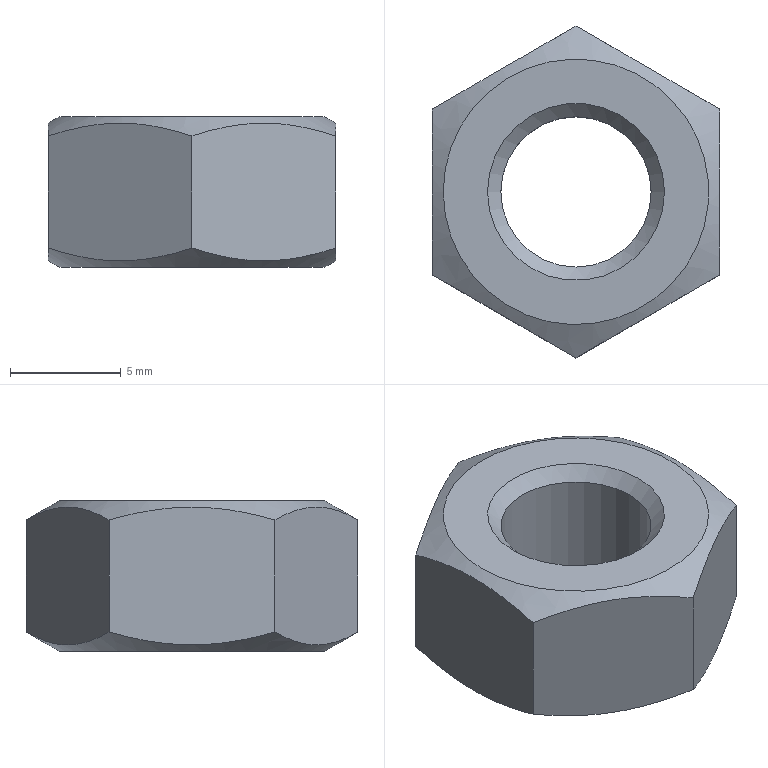Part | NX | features DATUM_CSYS 3, EXTRACT_DATUM_AXIS 2, EXTRACT_STRING 2, SKETCH 2, SWP104 2, EXTRUDE 1, HOLE PACKAGE 1, Instance Feature 1, Mirror Feature 1, SIMPLE HOLE 1, SYMBOLIC_THREAD 1 | 1 solid | 13 faces | box 12.99 x 15 x 6.8 mm | volume 720.374 mm3 | plane 8 | cone 4 | cylinder 1 | commonest cylinder face diameters 6.8 x1
STEP:
#1=CARTESIAN_POINT('',(-6.495,3.75,2.534));
#2=VERTEX_POINT('',#1);
#3=CARTESIAN_POINT('',(-6.495,3.75,-2.534));
#4=VERTEX_POINT('',#3);
#5=CARTESIAN_POINT('',(-6.495,3.75,3.4));
#6=DIRECTION('',(0.,0.,-1.));
#7=VECTOR('',#6,1000.);
#8=LINE('',#5,#7);
#9=EDGE_CURVE('',#2,#4,#8,.T.);
#10=ORIENTED_EDGE('',*,*,#9,.T.);
#11=CARTESIAN_POINT('',(-6.495,-3.75,-2.534));
#12=VERTEX_POINT('',#11);
#13=CARTESIAN_POINT('',(-6.495,-3.75,-2.534));
#14=CARTESIAN_POINT('',(-6.495,-2.53,-2.886));
#15=CARTESIAN_POINT('',(-6.495,-0.001629,-3.343));
#16=CARTESIAN_POINT('',(-6.495,2.538,-2.884));
#17=CARTESIAN_POINT('',(-6.495,3.75,-2.534));
#18=B_SPLINE_CURVE_WITH_KNOTS('',3,(#13,#14,#15,#16,#17),.UNSPECIFIED.,.F.,.F.,(4,1,4),(0.006647,0.01044,0.01424),.UNSPECIFIED.);
#19=EDGE_CURVE('',#4,#12,#18,.F.);
#20=ORIENTED_EDGE('',*,*,#19,.T.);
#21=CARTESIAN_POINT('',(-6.495,-3.75,2.534));
#22=VERTEX_POINT('',#21);
#23=CARTESIAN_POINT('',(-6.495,-3.75,3.4));
#24=DIRECTION('',(0.,0.,-1.));
#25=VECTOR('',#24,1000.);
#26=LINE('',#23,#25);
#27=EDGE_CURVE('',#22,#12,#26,.T.);
#28=ORIENTED_EDGE('',*,*,#27,.F.);
#29=CARTESIAN_POINT('',(-6.495,-3.75,2.534));
#30=CARTESIAN_POINT('',(-6.495,-2.53,2.886));
#31=CARTESIAN_POINT('',(-6.495,-0.001629,3.343));
#32=CARTESIAN_POINT('',(-6.495,2.538,2.884));
#33=CARTESIAN_POINT('',(-6.495,3.75,2.534));
#34=B_SPLINE_CURVE_WITH_KNOTS('',3,(#29,#30,#31,#32,#33),.UNSPECIFIED.,.F.,.F.,(4,1,4),(0.006647,0.01044,0.01424),.UNSPECIFIED.);
#35=EDGE_CURVE('',#22,#2,#34,.T.);
#36=ORIENTED_EDGE('',*,*,#35,.T.);
#37=EDGE_LOOP('',(#10,#20,#28,#36));
#38=FACE_BOUND('',#37,.T.);
#39=CARTESIAN_POINT('',(-6.495,3.75,3.4));
#40=DIRECTION('',(1.,0.,0.));
#41=DIRECTION('',(0.,1.,0.));
#42=AXIS2_PLACEMENT_3D('',#39,#40,#41);
#43=PLANE('',#42);
#44=ADVANCED_FACE('',(#38),#43,.F.);
#45=ORIENTED_EDGE('',*,*,#27,.T.);
#46=CARTESIAN_POINT('',(0.,-7.5,-2.534));
#47=VERTEX_POINT('',#46);
#48=CARTESIAN_POINT('',(-6.495,-3.75,-2.534));
#49=CARTESIAN_POINT('',(-5.435,-4.362,-2.887));
#50=CARTESIAN_POINT('',(-3.259,-5.618,-3.34));
#51=CARTESIAN_POINT('',(-1.062,-6.887,-2.888));
#52=CARTESIAN_POINT('',(0.,-7.5,-2.534));
#53=B_SPLINE_CURVE_WITH_KNOTS('',3,(#48,#49,#50,#51,#52),.UNSPECIFIED.,.F.,.F.,(4,1,4),(0.000000238,0.003788,0.007575),.UNSPECIFIED.);
#54=EDGE_CURVE('',#12,#47,#53,.T.);
#55=ORIENTED_EDGE('',*,*,#54,.T.);
#56=CARTESIAN_POINT('',(0.,-7.5,2.534));
#57=VERTEX_POINT('',#56);
#58=CARTESIAN_POINT('',(0.,-7.5,3.4));
#59=DIRECTION('',(0.,0.,-1.));
#60=VECTOR('',#59,1000.);
#61=LINE('',#58,#60);
#62=EDGE_CURVE('',#57,#47,#61,.T.);
#63=ORIENTED_EDGE('',*,*,#62,.F.);
#64=CARTESIAN_POINT('',(0.,-7.5,2.534));
#65=CARTESIAN_POINT('',(-1.061,-6.888,2.887));
#66=CARTESIAN_POINT('',(-3.236,-5.632,3.34));
#67=CARTESIAN_POINT('',(-5.433,-4.363,2.888));
#68=CARTESIAN_POINT('',(-6.495,-3.75,2.534));
#69=B_SPLINE_CURVE_WITH_KNOTS('',3,(#64,#65,#66,#67,#68),.UNSPECIFIED.,.F.,.F.,(4,1,4),(0.000000238,0.003788,0.007575),.UNSPECIFIED.);
#70=EDGE_CURVE('',#57,#22,#69,.T.);
#71=ORIENTED_EDGE('',*,*,#70,.T.);
#72=EDGE_LOOP('',(#45,#55,#63,#71));
#73=FACE_BOUND('',#72,.T.);
#74=CARTESIAN_POINT('',(-6.495,-3.75,3.4));
#75=DIRECTION('',(0.5,0.866,0.));
#76=DIRECTION('',(-0.866,0.5,0.));
#77=AXIS2_PLACEMENT_3D('',#74,#75,#76);
#78=PLANE('',#77);
#79=ADVANCED_FACE('',(#73),#78,.F.);
#80=ORIENTED_EDGE('',*,*,#62,.T.);
#81=CARTESIAN_POINT('',(6.495,-3.75,-2.534));
#82=VERTEX_POINT('',#81);
#83=CARTESIAN_POINT('',(0.,-7.5,-2.534));
#84=CARTESIAN_POINT('',(1.061,-6.888,-2.887));
#85=CARTESIAN_POINT('',(3.236,-5.632,-3.34));
#86=CARTESIAN_POINT('',(5.433,-4.363,-2.888));
#87=CARTESIAN_POINT('',(6.495,-3.75,-2.534));
#88=B_SPLINE_CURVE_WITH_KNOTS('',3,(#83,#84,#85,#86,#87),.UNSPECIFIED.,.F.,.F.,(4,1,4),(0.000000238,0.003788,0.007575),.UNSPECIFIED.);
#89=EDGE_CURVE('',#47,#82,#88,.T.);
#90=ORIENTED_EDGE('',*,*,#89,.T.);
#91=CARTESIAN_POINT('',(6.495,-3.75,2.534));
#92=VERTEX_POINT('',#91);
#93=CARTESIAN_POINT('',(6.495,-3.75,3.4));
#94=DIRECTION('',(0.,0.,-1.));
#95=VECTOR('',#94,1000.);
#96=LINE('',#93,#95);
#97=EDGE_CURVE('',#92,#82,#96,.T.);
#98=ORIENTED_EDGE('',*,*,#97,.F.);
#99=CARTESIAN_POINT('',(6.495,-3.75,2.534));
#100=CARTESIAN_POINT('',(5.435,-4.362,2.887));
#101=CARTESIAN_POINT('',(3.259,-5.618,3.34));
#102=CARTESIAN_POINT('',(1.062,-6.887,2.888));
#103=CARTESIAN_POINT('',(0.,-7.5,2.534));
#104=B_SPLINE_CURVE_WITH_KNOTS('',3,(#99,#100,#101,#102,#103),.UNSPECIFIED.,.F.,.F.,(4,1,4),(0.000000238,0.003788,0.007575),.UNSPECIFIED.);
#105=EDGE_CURVE('',#92,#57,#104,.T.);
#106=ORIENTED_EDGE('',*,*,#105,.T.);
#107=EDGE_LOOP('',(#80,#90,#98,#106));
#108=FACE_BOUND('',#107,.T.);
#109=CARTESIAN_POINT('',(0.,-7.5,3.4));
#110=DIRECTION('',(-0.5,0.866,0.));
#111=DIRECTION('',(-0.866,-0.5,0.));
#112=AXIS2_PLACEMENT_3D('',#109,#110,#111);
#113=PLANE('',#112);
#114=ADVANCED_FACE('',(#108),#113,.F.);
#115=ORIENTED_EDGE('',*,*,#97,.T.);
#116=CARTESIAN_POINT('',(6.495,3.75,-2.534));
#117=VERTEX_POINT('',#116);
#118=CARTESIAN_POINT('',(6.495,-3.75,-2.534));
#119=CARTESIAN_POINT('',(6.495,-2.53,-2.886));
#120=CARTESIAN_POINT('',(6.495,-0.001629,-3.343));
#121=CARTESIAN_POINT('',(6.495,2.538,-2.884));
#122=CARTESIAN_POINT('',(6.495,3.75,-2.534));
#123=B_SPLINE_CURVE_WITH_KNOTS('',3,(#118,#119,#120,#121,#122),.UNSPECIFIED.,.F.,.F.,(4,1,4),(0.006647,0.01044,0.01424),.UNSPECIFIED.);
#124=EDGE_CURVE('',#82,#117,#123,.T.);
#125=ORIENTED_EDGE('',*,*,#124,.T.);
#126=CARTESIAN_POINT('',(6.495,3.75,2.534));
#127=VERTEX_POINT('',#126);
#128=CARTESIAN_POINT('',(6.495,3.75,3.4));
#129=DIRECTION('',(0.,0.,-1.));
#130=VECTOR('',#129,1000.);
#131=LINE('',#128,#130);
#132=EDGE_CURVE('',#127,#117,#131,.T.);
#133=ORIENTED_EDGE('',*,*,#132,.F.);
#134=CARTESIAN_POINT('',(6.495,-3.75,2.534));
#135=CARTESIAN_POINT('',(6.495,-2.53,2.886));
#136=CARTESIAN_POINT('',(6.495,-0.001629,3.343));
#137=CARTESIAN_POINT('',(6.495,2.538,2.884));
#138=CARTESIAN_POINT('',(6.495,3.75,2.534));
#139=B_SPLINE_CURVE_WITH_KNOTS('',3,(#134,#135,#136,#137,#138),.UNSPECIFIED.,.F.,.F.,(4,1,4),(0.006647,0.01044,0.01424),.UNSPECIFIED.);
#140=EDGE_CURVE('',#127,#92,#139,.F.);
#141=ORIENTED_EDGE('',*,*,#140,.T.);
#142=EDGE_LOOP('',(#115,#125,#133,#141));
#143=FACE_BOUND('',#142,.T.);
#144=CARTESIAN_POINT('',(6.495,-3.75,3.4));
#145=DIRECTION('',(-1.,0.,0.));
#146=DIRECTION('',(0.,-1.,0.));
#147=AXIS2_PLACEMENT_3D('',#144,#145,#146);
#148=PLANE('',#147);
#149=ADVANCED_FACE('',(#143),#148,.F.);
#150=ORIENTED_EDGE('',*,*,#132,.T.);
#151=CARTESIAN_POINT('',(0.,7.5,-2.534));
#152=VERTEX_POINT('',#151);
#153=CARTESIAN_POINT('',(6.495,3.75,-2.534));
#154=CARTESIAN_POINT('',(5.435,4.362,-2.887));
#155=CARTESIAN_POINT('',(3.259,5.618,-3.34));
#156=CARTESIAN_POINT('',(1.062,6.887,-2.888));
#157=CARTESIAN_POINT('',(0.,7.5,-2.534));
#158=B_SPLINE_CURVE_WITH_KNOTS('',3,(#153,#154,#155,#156,#157),.UNSPECIFIED.,.F.,.F.,(4,1,4),(0.000000238,0.003788,0.007575),.UNSPECIFIED.);
#159=EDGE_CURVE('',#117,#152,#158,.T.);
#160=ORIENTED_EDGE('',*,*,#159,.T.);
#161=CARTESIAN_POINT('',(0.,7.5,2.534));
#162=VERTEX_POINT('',#161);
#163=CARTESIAN_POINT('',(0.,7.5,3.4));
#164=DIRECTION('',(0.,0.,-1.));
#165=VECTOR('',#164,1000.);
#166=LINE('',#163,#165);
#167=EDGE_CURVE('',#162,#152,#166,.T.);
#168=ORIENTED_EDGE('',*,*,#167,.F.);
#169=CARTESIAN_POINT('',(0.,7.5,2.534));
#170=CARTESIAN_POINT('',(1.061,6.888,2.887));
#171=CARTESIAN_POINT('',(3.236,5.632,3.34));
#172=CARTESIAN_POINT('',(5.433,4.363,2.888));
#173=CARTESIAN_POINT('',(6.495,3.75,2.534));
#174=B_SPLINE_CURVE_WITH_KNOTS('',3,(#169,#170,#171,#172,#173),.UNSPECIFIED.,.F.,.F.,(4,1,4),(0.000000238,0.003788,0.007575),.UNSPECIFIED.);
#175=EDGE_CURVE('',#162,#127,#174,.T.);
#176=ORIENTED_EDGE('',*,*,#175,.T.);
#177=EDGE_LOOP('',(#150,#160,#168,#176));
#178=FACE_BOUND('',#177,.T.);
#179=CARTESIAN_POINT('',(6.495,3.75,3.4));
#180=DIRECTION('',(-0.5,-0.866,0.));
#181=DIRECTION('',(0.866,-0.5,0.));
#182=AXIS2_PLACEMENT_3D('',#179,#180,#181);
#183=PLANE('',#182);
#184=ADVANCED_FACE('',(#178),#183,.F.);
#185=ORIENTED_EDGE('',*,*,#167,.T.);
#186=CARTESIAN_POINT('',(0.,7.5,-2.534));
#187=CARTESIAN_POINT('',(-1.061,6.888,-2.887));
#188=CARTESIAN_POINT('',(-3.236,5.632,-3.34));
#189=CARTESIAN_POINT('',(-5.433,4.363,-2.888));
#190=CARTESIAN_POINT('',(-6.495,3.75,-2.534));
#191=B_SPLINE_CURVE_WITH_KNOTS('',3,(#186,#187,#188,#189,#190),.UNSPECIFIED.,.F.,.F.,(4,1,4),(0.000000238,0.003788,0.007575),.UNSPECIFIED.);
#192=EDGE_CURVE('',#152,#4,#191,.T.);
#193=ORIENTED_EDGE('',*,*,#192,.T.);
#194=ORIENTED_EDGE('',*,*,#9,.F.);
#195=CARTESIAN_POINT('',(-6.495,3.75,2.534));
#196=CARTESIAN_POINT('',(-5.435,4.362,2.887));
#197=CARTESIAN_POINT('',(-3.259,5.618,3.34));
#198=CARTESIAN_POINT('',(-1.062,6.887,2.888));
#199=CARTESIAN_POINT('',(0.,7.5,2.534));
#200=B_SPLINE_CURVE_WITH_KNOTS('',3,(#195,#196,#197,#198,#199),.UNSPECIFIED.,.F.,.F.,(4,1,4),(0.000000238,0.003788,0.007575),.UNSPECIFIED.);
#201=EDGE_CURVE('',#2,#162,#200,.T.);
#202=ORIENTED_EDGE('',*,*,#201,.T.);
#203=EDGE_LOOP('',(#185,#193,#194,#202));
#204=FACE_BOUND('',#203,.T.);
#205=CARTESIAN_POINT('',(0.,7.5,3.4));
#206=DIRECTION('',(0.5,-0.866,0.));
#207=DIRECTION('',(0.866,0.5,0.));
#208=AXIS2_PLACEMENT_3D('',#205,#206,#207);
#209=PLANE('',#208);
#210=ADVANCED_FACE('',(#204),#209,.F.);
#211=CARTESIAN_POINT('',(-6.,0.,3.4));
#212=VERTEX_POINT('',#211);
#213=CARTESIAN_POINT('',(0.,0.,3.4));
#214=DIRECTION('',(0.,0.,-1.));
#215=DIRECTION('',(-1.,0.,0.));
#216=AXIS2_PLACEMENT_3D('',#213,#214,#215);
#217=CIRCLE('',#216,6.);
#218=EDGE_CURVE('',#212,#212,#217,.T.);
#219=ORIENTED_EDGE('',*,*,#218,.T.);
#220=EDGE_LOOP('',(#219));
#221=FACE_BOUND('',#220,.T.);
#222=ORIENTED_EDGE('',*,*,#70,.F.);
#223=ORIENTED_EDGE('',*,*,#105,.F.);
#224=ORIENTED_EDGE('',*,*,#140,.F.);
#225=ORIENTED_EDGE('',*,*,#175,.F.);
#226=ORIENTED_EDGE('',*,*,#201,.F.);
#227=ORIENTED_EDGE('',*,*,#35,.F.);
#228=EDGE_LOOP('',(#222,#223,#224,#225,#226,#227));
#229=FACE_BOUND('',#228,.T.);
#230=CARTESIAN_POINT('',(0.,0.,3.4));
#231=DIRECTION('',(0.,0.,-1.));
#232=DIRECTION('',(-1.,0.,0.));
#233=AXIS2_PLACEMENT_3D('',#230,#231,#232);
#234=CONICAL_SURFACE('',#233,6.,1.047);
#235=ADVANCED_FACE('',(#221,#229),#234,.T.);
#236=CARTESIAN_POINT('',(4.,0.,3.4));
#237=VERTEX_POINT('',#236);
#238=CARTESIAN_POINT('',(0.,0.,3.4));
#239=DIRECTION('',(0.,0.,1.));
#240=DIRECTION('',(1.,0.,0.));
#241=AXIS2_PLACEMENT_3D('',#238,#239,#240);
#242=CIRCLE('',#241,4.);
#243=EDGE_CURVE('',#237,#237,#242,.F.);
#244=ORIENTED_EDGE('',*,*,#243,.T.);
#245=EDGE_LOOP('',(#244));
#246=FACE_BOUND('',#245,.T.);
#247=ORIENTED_EDGE('',*,*,#218,.F.);
#248=EDGE_LOOP('',(#247));
#249=FACE_BOUND('',#248,.T.);
#250=CARTESIAN_POINT('',(0.,0.,3.4));
#251=DIRECTION('',(0.,0.,1.));
#252=DIRECTION('',(1.,0.,0.));
#253=AXIS2_PLACEMENT_3D('',#250,#251,#252);
#254=PLANE('',#253);
#255=ADVANCED_FACE('',(#246,#249),#254,.T.);
#256=CARTESIAN_POINT('',(6.,0.,-3.4));
#257=VERTEX_POINT('',#256);
#258=CARTESIAN_POINT('',(0.,0.,-3.4));
#259=DIRECTION('',(0.,0.,1.));
#260=DIRECTION('',(1.,0.,0.));
#261=AXIS2_PLACEMENT_3D('',#258,#259,#260);
#262=CIRCLE('',#261,6.);
#263=EDGE_CURVE('',#257,#257,#262,.T.);
#264=ORIENTED_EDGE('',*,*,#263,.T.);
#265=EDGE_LOOP('',(#264));
#266=FACE_BOUND('',#265,.T.);
#267=ORIENTED_EDGE('',*,*,#192,.F.);
#268=ORIENTED_EDGE('',*,*,#159,.F.);
#269=ORIENTED_EDGE('',*,*,#124,.F.);
#270=ORIENTED_EDGE('',*,*,#89,.F.);
#271=ORIENTED_EDGE('',*,*,#54,.F.);
#272=ORIENTED_EDGE('',*,*,#19,.F.);
#273=EDGE_LOOP('',(#267,#268,#269,#270,#271,#272));
#274=FACE_BOUND('',#273,.T.);
#275=CARTESIAN_POINT('',(0.,0.,-3.4));
#276=DIRECTION('',(0.,0.,1.));
#277=DIRECTION('',(1.,0.,0.));
#278=AXIS2_PLACEMENT_3D('',#275,#276,#277);
#279=CONICAL_SURFACE('',#278,6.,1.047);
#280=ADVANCED_FACE('',(#266,#274),#279,.T.);
#281=CARTESIAN_POINT('',(4.,0.,-3.4));
#282=VERTEX_POINT('',#281);
#283=CARTESIAN_POINT('',(0.,0.,-3.4));
#284=DIRECTION('',(0.,0.,1.));
#285=DIRECTION('',(1.,0.,0.));
#286=AXIS2_PLACEMENT_3D('',#283,#284,#285);
#287=CIRCLE('',#286,4.);
#288=EDGE_CURVE('',#282,#282,#287,.T.);
#289=ORIENTED_EDGE('',*,*,#288,.T.);
#290=EDGE_LOOP('',(#289));
#291=FACE_BOUND('',#290,.T.);
#292=ORIENTED_EDGE('',*,*,#263,.F.);
#293=EDGE_LOOP('',(#292));
#294=FACE_BOUND('',#293,.T.);
#295=CARTESIAN_POINT('',(0.,0.,-3.4));
#296=DIRECTION('',(0.,0.,1.));
#297=DIRECTION('',(1.,0.,0.));
#298=AXIS2_PLACEMENT_3D('',#295,#296,#297);
#299=PLANE('',#298);
#300=ADVANCED_FACE('',(#291,#294),#299,.F.);
#301=CARTESIAN_POINT('',(3.4,0.,-2.8));
#302=VERTEX_POINT('',#301);
#303=CARTESIAN_POINT('',(0.,0.,-2.8));
#304=DIRECTION('',(0.,0.,1.));
#305=DIRECTION('',(1.,0.,0.));
#306=AXIS2_PLACEMENT_3D('',#303,#304,#305);
#307=CIRCLE('',#306,3.4);
#308=EDGE_CURVE('',#302,#302,#307,.F.);
#309=ORIENTED_EDGE('',*,*,#308,.T.);
#310=EDGE_LOOP('',(#309));
#311=FACE_BOUND('',#310,.T.);
#312=CARTESIAN_POINT('',(3.4,0.,2.8));
#313=VERTEX_POINT('',#312);
#314=CARTESIAN_POINT('',(0.,0.,2.8));
#315=DIRECTION('',(0.,0.,1.));
#316=DIRECTION('',(1.,0.,0.));
#317=AXIS2_PLACEMENT_3D('',#314,#315,#316);
#318=CIRCLE('',#317,3.4);
#319=EDGE_CURVE('',#313,#313,#318,.T.);
#320=ORIENTED_EDGE('',*,*,#319,.T.);
#321=EDGE_LOOP('',(#320));
#322=FACE_BOUND('',#321,.T.);
#323=CARTESIAN_POINT('',(0.,0.,3.4));
#324=DIRECTION('',(0.,0.,-1.));
#325=DIRECTION('',(-1.,0.,0.));
#326=AXIS2_PLACEMENT_3D('',#323,#324,#325);
#327=CYLINDRICAL_SURFACE('',#326,3.4);
#328=ADVANCED_FACE('',(#311,#322),#327,.F.);
#329=ORIENTED_EDGE('',*,*,#319,.F.);
#330=EDGE_LOOP('',(#329));
#331=FACE_BOUND('',#330,.T.);
#332=ORIENTED_EDGE('',*,*,#243,.F.);
#333=EDGE_LOOP('',(#332));
#334=FACE_BOUND('',#333,.T.);
#335=CARTESIAN_POINT('',(0.,0.,3.4));
#336=DIRECTION('',(0.,0.,1.));
#337=DIRECTION('',(1.,0.,0.));
#338=AXIS2_PLACEMENT_3D('',#335,#336,#337);
#339=CONICAL_SURFACE('',#338,4.,0.7854);
#340=ADVANCED_FACE('',(#331,#334),#339,.F.);
#341=ORIENTED_EDGE('',*,*,#308,.F.);
#342=EDGE_LOOP('',(#341));
#343=FACE_BOUND('',#342,.T.);
#344=ORIENTED_EDGE('',*,*,#288,.F.);
#345=EDGE_LOOP('',(#344));
#346=FACE_BOUND('',#345,.T.);
#347=CARTESIAN_POINT('',(0.,0.,-3.4));
#348=DIRECTION('',(0.,0.,-1.));
#349=DIRECTION('',(-1.,0.,0.));
#350=AXIS2_PLACEMENT_3D('',#347,#348,#349);
#351=CONICAL_SURFACE('',#350,4.,0.7854);
#352=ADVANCED_FACE('',(#343,#346),#351,.F.);
#353=CLOSED_SHELL('',(#44,#79,#114,#149,#184,#210,#235,#255,#280,#300,#328,#340,#352));
#354=MANIFOLD_SOLID_BREP('',#353);
#355=(LENGTH_UNIT()NAMED_UNIT(*)SI_UNIT(.MILLI.,.METRE.));
#356=UNCERTAINTY_MEASURE_WITH_UNIT(LENGTH_MEASURE(0.0508),#355,'','');
#357=(NAMED_UNIT(*)PLANE_ANGLE_UNIT()SI_UNIT($,.RADIAN.));
#358=(NAMED_UNIT(*)SI_UNIT($,.STERADIAN.)SOLID_ANGLE_UNIT());
#359=(GEOMETRIC_REPRESENTATION_CONTEXT(3)GLOBAL_UNCERTAINTY_ASSIGNED_CONTEXT((#356))GLOBAL_UNIT_ASSIGNED_CONTEXT((#355,#357,#358))REPRESENTATION_CONTEXT('',''));
#360=ADVANCED_BREP_SHAPE_REPRESENTATION('',(#354),#359);